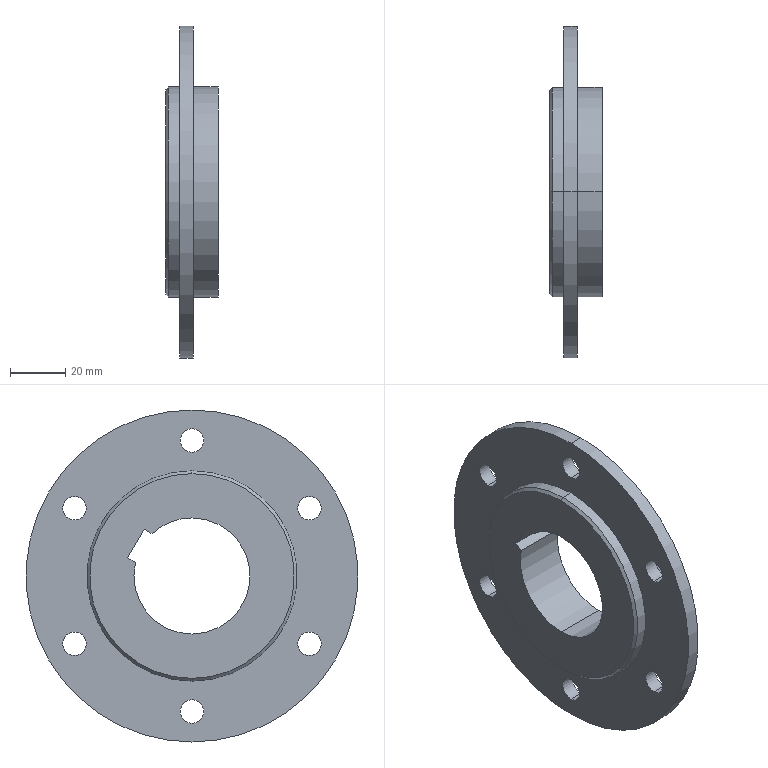Part | SolidWorks | features Chamfer 1, Extrusion 1, HoleWzd 1, ICE 1 | 1 solid | 30 faces | box 19 x 120 x 120 mm | volume 91296 mm3 | cylinder 21 | plane 7 | cone 2 | commonest cylinder face diameters 8.5 x12 76 x4 42 x3 120 x2
STEP:
#1=CARTESIAN_POINT('',(5.,42.435,28.75));
#2=VERTEX_POINT('',#1);
#3=CARTESIAN_POINT('',(5.,42.435,20.25));
#4=VERTEX_POINT('',#3);
#5=CARTESIAN_POINT('',(5.,42.435,24.5));
#6=DIRECTION('',(1.,0.,0.));
#7=DIRECTION('',(0.,0.,-1.));
#8=AXIS2_PLACEMENT_3D('',#5,#6,#7);
#9=CIRCLE('',#8,4.25);
#10=EDGE_CURVE('',#2,#4,#9,.T.);
#11=ORIENTED_EDGE('',*,*,#10,.T.);
#12=CARTESIAN_POINT('',(0.,42.435,20.25));
#13=VERTEX_POINT('',#12);
#14=CARTESIAN_POINT('',(0.,42.435,20.25));
#15=DIRECTION('',(-1.,0.,0.));
#16=VECTOR('',#15,1000.);
#17=LINE('',#14,#16);
#18=EDGE_CURVE('',#4,#13,#17,.T.);
#19=ORIENTED_EDGE('',*,*,#18,.T.);
#20=CARTESIAN_POINT('',(0.,42.435,28.75));
#21=VERTEX_POINT('',#20);
#22=CARTESIAN_POINT('',(0.,42.435,24.5));
#23=DIRECTION('',(-1.,0.,0.));
#24=DIRECTION('',(0.,0.,1.));
#25=AXIS2_PLACEMENT_3D('',#22,#23,#24);
#26=CIRCLE('',#25,4.25);
#27=EDGE_CURVE('',#13,#21,#26,.T.);
#28=ORIENTED_EDGE('',*,*,#27,.T.);
#29=CARTESIAN_POINT('',(0.,42.435,28.75));
#30=DIRECTION('',(-1.,0.,0.));
#31=VECTOR('',#30,1000.);
#32=LINE('',#29,#31);
#33=EDGE_CURVE('',#2,#21,#32,.T.);
#34=ORIENTED_EDGE('',*,*,#33,.F.);
#35=EDGE_LOOP('',(#11,#19,#28,#34));
#36=FACE_OUTER_BOUND('',#35,.T.);
#37=CARTESIAN_POINT('',(0.,42.435,24.5));
#38=DIRECTION('',(-1.,0.,0.));
#39=DIRECTION('',(0.,0.,1.));
#40=AXIS2_PLACEMENT_3D('',#37,#38,#39);
#41=CYLINDRICAL_SURFACE('',#40,4.25);
#42=ADVANCED_FACE('',(#36),#41,.F.);
#43=CARTESIAN_POINT('',(5.,0.,53.25));
#44=VERTEX_POINT('',#43);
#45=CARTESIAN_POINT('',(5.,0.,44.75));
#46=VERTEX_POINT('',#45);
#47=CARTESIAN_POINT('',(5.,0.,49.));
#48=DIRECTION('',(1.,0.,0.));
#49=DIRECTION('',(0.,0.,-1.));
#50=AXIS2_PLACEMENT_3D('',#47,#48,#49);
#51=CIRCLE('',#50,4.25);
#52=EDGE_CURVE('',#44,#46,#51,.T.);
#53=ORIENTED_EDGE('',*,*,#52,.T.);
#54=CARTESIAN_POINT('',(0.,0.,44.75));
#55=VERTEX_POINT('',#54);
#56=CARTESIAN_POINT('',(0.,0.,44.75));
#57=DIRECTION('',(-1.,0.,0.));
#58=VECTOR('',#57,1000.);
#59=LINE('',#56,#58);
#60=EDGE_CURVE('',#46,#55,#59,.T.);
#61=ORIENTED_EDGE('',*,*,#60,.T.);
#62=CARTESIAN_POINT('',(0.,0.,53.25));
#63=VERTEX_POINT('',#62);
#64=CARTESIAN_POINT('',(0.,0.,49.));
#65=DIRECTION('',(-1.,0.,0.));
#66=DIRECTION('',(0.,0.,1.));
#67=AXIS2_PLACEMENT_3D('',#64,#65,#66);
#68=CIRCLE('',#67,4.25);
#69=EDGE_CURVE('',#55,#63,#68,.T.);
#70=ORIENTED_EDGE('',*,*,#69,.T.);
#71=CARTESIAN_POINT('',(0.,0.,53.25));
#72=DIRECTION('',(-1.,0.,0.));
#73=VECTOR('',#72,1000.);
#74=LINE('',#71,#73);
#75=EDGE_CURVE('',#44,#63,#74,.T.);
#76=ORIENTED_EDGE('',*,*,#75,.F.);
#77=EDGE_LOOP('',(#53,#61,#70,#76));
#78=FACE_OUTER_BOUND('',#77,.T.);
#79=CARTESIAN_POINT('',(0.,0.,49.));
#80=DIRECTION('',(-1.,0.,0.));
#81=DIRECTION('',(0.,0.,1.));
#82=AXIS2_PLACEMENT_3D('',#79,#80,#81);
#83=CYLINDRICAL_SURFACE('',#82,4.25);
#84=ADVANCED_FACE('',(#78),#83,.F.);
#85=CARTESIAN_POINT('',(5.,-42.435,28.75));
#86=VERTEX_POINT('',#85);
#87=CARTESIAN_POINT('',(5.,-42.435,20.25));
#88=VERTEX_POINT('',#87);
#89=CARTESIAN_POINT('',(5.,-42.435,24.5));
#90=DIRECTION('',(1.,0.,0.));
#91=DIRECTION('',(0.,0.,-1.));
#92=AXIS2_PLACEMENT_3D('',#89,#90,#91);
#93=CIRCLE('',#92,4.25);
#94=EDGE_CURVE('',#86,#88,#93,.T.);
#95=ORIENTED_EDGE('',*,*,#94,.T.);
#96=CARTESIAN_POINT('',(0.,-42.435,20.25));
#97=VERTEX_POINT('',#96);
#98=CARTESIAN_POINT('',(0.,-42.435,20.25));
#99=DIRECTION('',(-1.,0.,0.));
#100=VECTOR('',#99,1000.);
#101=LINE('',#98,#100);
#102=EDGE_CURVE('',#88,#97,#101,.T.);
#103=ORIENTED_EDGE('',*,*,#102,.T.);
#104=CARTESIAN_POINT('',(0.,-42.435,28.75));
#105=VERTEX_POINT('',#104);
#106=CARTESIAN_POINT('',(0.,-42.435,24.5));
#107=DIRECTION('',(-1.,0.,0.));
#108=DIRECTION('',(0.,0.,1.));
#109=AXIS2_PLACEMENT_3D('',#106,#107,#108);
#110=CIRCLE('',#109,4.25);
#111=EDGE_CURVE('',#97,#105,#110,.T.);
#112=ORIENTED_EDGE('',*,*,#111,.T.);
#113=CARTESIAN_POINT('',(0.,-42.435,28.75));
#114=DIRECTION('',(-1.,0.,0.));
#115=VECTOR('',#114,1000.);
#116=LINE('',#113,#115);
#117=EDGE_CURVE('',#86,#105,#116,.T.);
#118=ORIENTED_EDGE('',*,*,#117,.F.);
#119=EDGE_LOOP('',(#95,#103,#112,#118));
#120=FACE_OUTER_BOUND('',#119,.T.);
#121=CARTESIAN_POINT('',(0.,-42.435,24.5));
#122=DIRECTION('',(-1.,0.,0.));
#123=DIRECTION('',(0.,0.,1.));
#124=AXIS2_PLACEMENT_3D('',#121,#122,#123);
#125=CYLINDRICAL_SURFACE('',#124,4.25);
#126=ADVANCED_FACE('',(#120),#125,.F.);
#127=CARTESIAN_POINT('',(5.,-42.435,-20.25));
#128=VERTEX_POINT('',#127);
#129=CARTESIAN_POINT('',(5.,-42.435,-28.75));
#130=VERTEX_POINT('',#129);
#131=CARTESIAN_POINT('',(5.,-42.435,-24.5));
#132=DIRECTION('',(1.,0.,0.));
#133=DIRECTION('',(0.,0.,-1.));
#134=AXIS2_PLACEMENT_3D('',#131,#132,#133);
#135=CIRCLE('',#134,4.25);
#136=EDGE_CURVE('',#128,#130,#135,.T.);
#137=ORIENTED_EDGE('',*,*,#136,.T.);
#138=CARTESIAN_POINT('',(0.,-42.435,-28.75));
#139=VERTEX_POINT('',#138);
#140=CARTESIAN_POINT('',(0.,-42.435,-28.75));
#141=DIRECTION('',(-1.,0.,0.));
#142=VECTOR('',#141,1000.);
#143=LINE('',#140,#142);
#144=EDGE_CURVE('',#130,#139,#143,.T.);
#145=ORIENTED_EDGE('',*,*,#144,.T.);
#146=CARTESIAN_POINT('',(0.,-42.435,-20.25));
#147=VERTEX_POINT('',#146);
#148=CARTESIAN_POINT('',(0.,-42.435,-24.5));
#149=DIRECTION('',(-1.,0.,0.));
#150=DIRECTION('',(0.,0.,1.));
#151=AXIS2_PLACEMENT_3D('',#148,#149,#150);
#152=CIRCLE('',#151,4.25);
#153=EDGE_CURVE('',#139,#147,#152,.T.);
#154=ORIENTED_EDGE('',*,*,#153,.T.);
#155=CARTESIAN_POINT('',(0.,-42.435,-20.25));
#156=DIRECTION('',(-1.,0.,0.));
#157=VECTOR('',#156,1000.);
#158=LINE('',#155,#157);
#159=EDGE_CURVE('',#128,#147,#158,.T.);
#160=ORIENTED_EDGE('',*,*,#159,.F.);
#161=EDGE_LOOP('',(#137,#145,#154,#160));
#162=FACE_OUTER_BOUND('',#161,.T.);
#163=CARTESIAN_POINT('',(0.,-42.435,-24.5));
#164=DIRECTION('',(-1.,0.,0.));
#165=DIRECTION('',(0.,0.,1.));
#166=AXIS2_PLACEMENT_3D('',#163,#164,#165);
#167=CYLINDRICAL_SURFACE('',#166,4.25);
#168=ADVANCED_FACE('',(#162),#167,.F.);
#169=CARTESIAN_POINT('',(5.,0.,-44.75));
#170=VERTEX_POINT('',#169);
#171=CARTESIAN_POINT('',(5.,0.,-53.25));
#172=VERTEX_POINT('',#171);
#173=CARTESIAN_POINT('',(5.,0.,-49.));
#174=DIRECTION('',(1.,0.,0.));
#175=DIRECTION('',(0.,0.,-1.));
#176=AXIS2_PLACEMENT_3D('',#173,#174,#175);
#177=CIRCLE('',#176,4.25);
#178=EDGE_CURVE('',#170,#172,#177,.T.);
#179=ORIENTED_EDGE('',*,*,#178,.T.);
#180=CARTESIAN_POINT('',(0.,0.,-53.25));
#181=VERTEX_POINT('',#180);
#182=CARTESIAN_POINT('',(0.,0.,-53.25));
#183=DIRECTION('',(-1.,0.,0.));
#184=VECTOR('',#183,1000.);
#185=LINE('',#182,#184);
#186=EDGE_CURVE('',#172,#181,#185,.T.);
#187=ORIENTED_EDGE('',*,*,#186,.T.);
#188=CARTESIAN_POINT('',(0.,0.,-44.75));
#189=VERTEX_POINT('',#188);
#190=CARTESIAN_POINT('',(0.,0.,-49.));
#191=DIRECTION('',(-1.,0.,0.));
#192=DIRECTION('',(0.,0.,1.));
#193=AXIS2_PLACEMENT_3D('',#190,#191,#192);
#194=CIRCLE('',#193,4.25);
#195=EDGE_CURVE('',#181,#189,#194,.T.);
#196=ORIENTED_EDGE('',*,*,#195,.T.);
#197=CARTESIAN_POINT('',(0.,0.,-44.75));
#198=DIRECTION('',(-1.,0.,0.));
#199=VECTOR('',#198,1000.);
#200=LINE('',#197,#199);
#201=EDGE_CURVE('',#170,#189,#200,.T.);
#202=ORIENTED_EDGE('',*,*,#201,.F.);
#203=EDGE_LOOP('',(#179,#187,#196,#202));
#204=FACE_OUTER_BOUND('',#203,.T.);
#205=CARTESIAN_POINT('',(0.,0.,-49.));
#206=DIRECTION('',(-1.,0.,0.));
#207=DIRECTION('',(0.,0.,1.));
#208=AXIS2_PLACEMENT_3D('',#205,#206,#207);
#209=CYLINDRICAL_SURFACE('',#208,4.25);
#210=ADVANCED_FACE('',(#204),#209,.F.);
#211=CARTESIAN_POINT('',(5.,42.435,-20.25));
#212=VERTEX_POINT('',#211);
#213=CARTESIAN_POINT('',(5.,42.435,-28.75));
#214=VERTEX_POINT('',#213);
#215=CARTESIAN_POINT('',(5.,42.435,-24.5));
#216=DIRECTION('',(1.,0.,0.));
#217=DIRECTION('',(0.,0.,-1.));
#218=AXIS2_PLACEMENT_3D('',#215,#216,#217);
#219=CIRCLE('',#218,4.25);
#220=EDGE_CURVE('',#212,#214,#219,.T.);
#221=ORIENTED_EDGE('',*,*,#220,.T.);
#222=CARTESIAN_POINT('',(0.,42.435,-28.75));
#223=VERTEX_POINT('',#222);
#224=CARTESIAN_POINT('',(0.,42.435,-28.75));
#225=DIRECTION('',(-1.,0.,0.));
#226=VECTOR('',#225,1000.);
#227=LINE('',#224,#226);
#228=EDGE_CURVE('',#214,#223,#227,.T.);
#229=ORIENTED_EDGE('',*,*,#228,.T.);
#230=CARTESIAN_POINT('',(0.,42.435,-20.25));
#231=VERTEX_POINT('',#230);
#232=CARTESIAN_POINT('',(0.,42.435,-24.5));
#233=DIRECTION('',(-1.,0.,0.));
#234=DIRECTION('',(0.,0.,1.));
#235=AXIS2_PLACEMENT_3D('',#232,#233,#234);
#236=CIRCLE('',#235,4.25);
#237=EDGE_CURVE('',#223,#231,#236,.T.);
#238=ORIENTED_EDGE('',*,*,#237,.T.);
#239=CARTESIAN_POINT('',(0.,42.435,-20.25));
#240=DIRECTION('',(-1.,0.,0.));
#241=VECTOR('',#240,1000.);
#242=LINE('',#239,#241);
#243=EDGE_CURVE('',#212,#231,#242,.T.);
#244=ORIENTED_EDGE('',*,*,#243,.F.);
#245=EDGE_LOOP('',(#221,#229,#238,#244));
#246=FACE_OUTER_BOUND('',#245,.T.);
#247=CARTESIAN_POINT('',(0.,42.435,-24.5));
#248=DIRECTION('',(-1.,0.,0.));
#249=DIRECTION('',(0.,0.,1.));
#250=AXIS2_PLACEMENT_3D('',#247,#248,#249);
#251=CYLINDRICAL_SURFACE('',#250,4.25);
#252=ADVANCED_FACE('',(#246),#251,.F.);
#253=CARTESIAN_POINT('',(-5.,0.,37.));
#254=VERTEX_POINT('',#253);
#255=CARTESIAN_POINT('',(-5.,0.,-37.));
#256=VERTEX_POINT('',#255);
#257=CARTESIAN_POINT('',(-5.,0.,0.));
#258=DIRECTION('',(-1.,0.,0.));
#259=DIRECTION('',(0.,0.,-1.));
#260=AXIS2_PLACEMENT_3D('',#257,#258,#259);
#261=CIRCLE('',#260,37.);
#262=EDGE_CURVE('',#254,#256,#261,.T.);
#263=ORIENTED_EDGE('',*,*,#262,.F.);
#264=CARTESIAN_POINT('',(-4.,0.,38.));
#265=VERTEX_POINT('',#264);
#266=CARTESIAN_POINT('',(-4.,0.,38.));
#267=DIRECTION('',(0.7071,0.,0.7071));
#268=VECTOR('',#267,1000.);
#269=LINE('',#266,#268);
#270=EDGE_CURVE('',#254,#265,#269,.T.);
#271=ORIENTED_EDGE('',*,*,#270,.T.);
#272=CARTESIAN_POINT('',(-4.,0.,-38.));
#273=VERTEX_POINT('',#272);
#274=CARTESIAN_POINT('',(-4.,0.,0.));
#275=DIRECTION('',(1.,0.,0.));
#276=DIRECTION('',(0.,0.,-1.));
#277=AXIS2_PLACEMENT_3D('',#274,#275,#276);
#278=CIRCLE('',#277,38.);
#279=EDGE_CURVE('',#273,#265,#278,.T.);
#280=ORIENTED_EDGE('',*,*,#279,.F.);
#281=CARTESIAN_POINT('',(-4.,0.,-38.));
#282=DIRECTION('',(0.7071,0.,-0.7071));
#283=VECTOR('',#282,1000.);
#284=LINE('',#281,#283);
#285=EDGE_CURVE('',#256,#273,#284,.T.);
#286=ORIENTED_EDGE('',*,*,#285,.F.);
#287=EDGE_LOOP('',(#263,#271,#280,#286));
#288=FACE_OUTER_BOUND('',#287,.T.);
#289=CARTESIAN_POINT('',(-4.,0.,0.));
#290=DIRECTION('',(1.,0.,0.));
#291=DIRECTION('',(0.,0.,-1.));
#292=AXIS2_PLACEMENT_3D('',#289,#290,#291);
#293=CONICAL_SURFACE('',#292,38.,0.7854);
#294=ADVANCED_FACE('',(#288),#293,.T.);
#295=CARTESIAN_POINT('',(5.,0.,-60.));
#296=VERTEX_POINT('',#295);
#297=CARTESIAN_POINT('',(5.,0.,60.));
#298=VERTEX_POINT('',#297);
#299=CARTESIAN_POINT('',(5.,0.,0.));
#300=DIRECTION('',(1.,0.,0.));
#301=DIRECTION('',(0.,0.,-1.));
#302=AXIS2_PLACEMENT_3D('',#299,#300,#301);
#303=CIRCLE('',#302,60.);
#304=EDGE_CURVE('',#296,#298,#303,.T.);
#305=ORIENTED_EDGE('',*,*,#304,.F.);
#306=CARTESIAN_POINT('',(0.,0.,-60.));
#307=VERTEX_POINT('',#306);
#308=CARTESIAN_POINT('',(5.,0.,-60.));
#309=DIRECTION('',(-1.,0.,0.));
#310=VECTOR('',#309,1000.);
#311=LINE('',#308,#310);
#312=EDGE_CURVE('',#296,#307,#311,.T.);
#313=ORIENTED_EDGE('',*,*,#312,.T.);
#314=CARTESIAN_POINT('',(0.,0.,60.));
#315=VERTEX_POINT('',#314);
#316=CARTESIAN_POINT('',(0.,0.,0.));
#317=DIRECTION('',(1.,0.,0.));
#318=DIRECTION('',(0.,0.,-1.));
#319=AXIS2_PLACEMENT_3D('',#316,#317,#318);
#320=CIRCLE('',#319,60.);
#321=EDGE_CURVE('',#307,#315,#320,.T.);
#322=ORIENTED_EDGE('',*,*,#321,.T.);
#323=CARTESIAN_POINT('',(5.,0.,60.));
#324=DIRECTION('',(-1.,0.,0.));
#325=VECTOR('',#324,1000.);
#326=LINE('',#323,#325);
#327=EDGE_CURVE('',#298,#315,#326,.T.);
#328=ORIENTED_EDGE('',*,*,#327,.F.);
#329=EDGE_LOOP('',(#305,#313,#322,#328));
#330=FACE_OUTER_BOUND('',#329,.T.);
#331=CARTESIAN_POINT('',(5.,0.,0.));
#332=DIRECTION('',(-1.,0.,0.));
#333=DIRECTION('',(0.,0.,1.));
#334=AXIS2_PLACEMENT_3D('',#331,#332,#333);
#335=CYLINDRICAL_SURFACE('',#334,60.);
#336=ADVANCED_FACE('',(#330),#335,.T.);
#337=CARTESIAN_POINT('',(-5.,0.,21.));
#338=VERTEX_POINT('',#337);
#339=CARTESIAN_POINT('',(-5.,0.,-21.));
#340=VERTEX_POINT('',#339);
#341=CARTESIAN_POINT('',(-5.,0.,0.));
#342=DIRECTION('',(1.,0.,0.));
#343=DIRECTION('',(0.,0.,-1.));
#344=AXIS2_PLACEMENT_3D('',#341,#342,#343);
#345=CIRCLE('',#344,21.);
#346=EDGE_CURVE('',#338,#340,#345,.T.);
#347=ORIENTED_EDGE('',*,*,#346,.F.);
#348=CARTESIAN_POINT('',(14.,0.,21.));
#349=VERTEX_POINT('',#348);
#350=CARTESIAN_POINT('',(-5.,0.,21.));
#351=DIRECTION('',(1.,0.,0.));
#352=VECTOR('',#351,1000.);
#353=LINE('',#350,#352);
#354=EDGE_CURVE('',#338,#349,#353,.T.);
#355=ORIENTED_EDGE('',*,*,#354,.T.);
#356=CARTESIAN_POINT('',(14.,0.,-21.));
#357=VERTEX_POINT('',#356);
#358=CARTESIAN_POINT('',(14.,0.,0.));
#359=DIRECTION('',(1.,0.,0.));
#360=DIRECTION('',(0.,0.,-1.));
#361=AXIS2_PLACEMENT_3D('',#358,#359,#360);
#362=CIRCLE('',#361,21.);
#363=EDGE_CURVE('',#349,#357,#362,.T.);
#364=ORIENTED_EDGE('',*,*,#363,.T.);
#365=CARTESIAN_POINT('',(-5.,0.,-21.));
#366=DIRECTION('',(1.,0.,0.));
#367=VECTOR('',#366,1000.);
#368=LINE('',#365,#367);
#369=EDGE_CURVE('',#340,#357,#368,.T.);
#370=ORIENTED_EDGE('',*,*,#369,.F.);
#371=EDGE_LOOP('',(#347,#355,#364,#370));
#372=FACE_OUTER_BOUND('',#371,.T.);
#373=CARTESIAN_POINT('',(-5.,0.,0.));
#374=DIRECTION('',(1.,0.,0.));
#375=DIRECTION('',(0.,0.,-1.));
#376=AXIS2_PLACEMENT_3D('',#373,#374,#375);
#377=CYLINDRICAL_SURFACE('',#376,21.);
#378=ADVANCED_FACE('',(#372),#377,.F.);
#379=CARTESIAN_POINT('',(-5.,20.428,4.866));
#380=VERTEX_POINT('',#379);
#381=CARTESIAN_POINT('',(-5.,0.,0.));
#382=DIRECTION('',(1.,0.,0.));
#383=DIRECTION('',(0.,0.,-1.));
#384=AXIS2_PLACEMENT_3D('',#381,#382,#383);
#385=CIRCLE('',#384,21.);
#386=EDGE_CURVE('',#340,#380,#385,.T.);
#387=ORIENTED_EDGE('',*,*,#386,.F.);
#388=ORIENTED_EDGE('',*,*,#369,.T.);
#389=CARTESIAN_POINT('',(14.,20.428,4.866));
#390=VERTEX_POINT('',#389);
#391=CARTESIAN_POINT('',(14.,0.,0.));
#392=DIRECTION('',(1.,0.,0.));
#393=DIRECTION('',(0.,0.,-1.));
#394=AXIS2_PLACEMENT_3D('',#391,#392,#393);
#395=CIRCLE('',#394,21.);
#396=EDGE_CURVE('',#357,#390,#395,.T.);
#397=ORIENTED_EDGE('',*,*,#396,.T.);
#398=CARTESIAN_POINT('',(-5.,20.428,4.866));
#399=DIRECTION('',(1.,0.,0.));
#400=VECTOR('',#399,1000.);
#401=LINE('',#398,#400);
#402=EDGE_CURVE('',#380,#390,#401,.T.);
#403=ORIENTED_EDGE('',*,*,#402,.F.);
#404=EDGE_LOOP('',(#387,#388,#397,#403));
#405=FACE_OUTER_BOUND('',#404,.T.);
#406=CARTESIAN_POINT('',(-5.,0.,0.));
#407=DIRECTION('',(1.,0.,0.));
#408=DIRECTION('',(0.,0.,-1.));
#409=AXIS2_PLACEMENT_3D('',#406,#407,#408);
#410=CYLINDRICAL_SURFACE('',#409,21.);
#411=ADVANCED_FACE('',(#405),#410,.F.);
#412=CARTESIAN_POINT('',(5.,0.,38.));
#413=VERTEX_POINT('',#412);
#414=CARTESIAN_POINT('',(5.,0.,-38.));
#415=VERTEX_POINT('',#414);
#416=CARTESIAN_POINT('',(5.,0.,0.));
#417=DIRECTION('',(-1.,0.,0.));
#418=DIRECTION('',(0.,0.,-1.));
#419=AXIS2_PLACEMENT_3D('',#416,#417,#418);
#420=CIRCLE('',#419,38.);
#421=EDGE_CURVE('',#413,#415,#420,.T.);
#422=ORIENTED_EDGE('',*,*,#421,.F.);
#423=CARTESIAN_POINT('',(14.,0.,38.));
#424=VERTEX_POINT('',#423);
#425=CARTESIAN_POINT('',(-5.,0.,38.));
#426=DIRECTION('',(1.,0.,0.));
#427=VECTOR('',#426,1000.);
#428=LINE('',#425,#427);
#429=EDGE_CURVE('',#413,#424,#428,.T.);
#430=ORIENTED_EDGE('',*,*,#429,.T.);
#431=CARTESIAN_POINT('',(14.,0.,-38.));
#432=VERTEX_POINT('',#431);
#433=CARTESIAN_POINT('',(14.,0.,0.));
#434=DIRECTION('',(1.,0.,0.));
#435=DIRECTION('',(0.,0.,-1.));
#436=AXIS2_PLACEMENT_3D('',#433,#434,#435);
#437=CIRCLE('',#436,38.);
#438=EDGE_CURVE('',#432,#424,#437,.T.);
#439=ORIENTED_EDGE('',*,*,#438,.F.);
#440=CARTESIAN_POINT('',(-5.,0.,-38.));
#441=DIRECTION('',(1.,0.,0.));
#442=VECTOR('',#441,1000.);
#443=LINE('',#440,#442);
#444=EDGE_CURVE('',#415,#432,#443,.T.);
#445=ORIENTED_EDGE('',*,*,#444,.F.);
#446=EDGE_LOOP('',(#422,#430,#439,#445));
#447=FACE_OUTER_BOUND('',#446,.T.);
#448=CARTESIAN_POINT('',(-5.,0.,0.));
#449=DIRECTION('',(1.,0.,0.));
#450=DIRECTION('',(0.,0.,-1.));
#451=AXIS2_PLACEMENT_3D('',#448,#449,#450);
#452=CYLINDRICAL_SURFACE('',#451,38.);
#453=ADVANCED_FACE('',(#447),#452,.T.);
#454=ORIENTED_EDGE('',*,*,#279,.T.);
#455=CARTESIAN_POINT('',(0.,0.,38.));
#456=VERTEX_POINT('',#455);
#457=CARTESIAN_POINT('',(-5.,0.,38.));
#458=DIRECTION('',(1.,0.,0.));
#459=VECTOR('',#458,1000.);
#460=LINE('',#457,#459);
#461=EDGE_CURVE('',#265,#456,#460,.T.);
#462=ORIENTED_EDGE('',*,*,#461,.T.);
#463=CARTESIAN_POINT('',(0.,0.,-38.));
#464=VERTEX_POINT('',#463);
#465=CARTESIAN_POINT('',(0.,0.,0.));
#466=DIRECTION('',(1.,0.,0.));
#467=DIRECTION('',(0.,0.,-1.));
#468=AXIS2_PLACEMENT_3D('',#465,#466,#467);
#469=CIRCLE('',#468,38.);
#470=EDGE_CURVE('',#464,#456,#469,.T.);
#471=ORIENTED_EDGE('',*,*,#470,.F.);
#472=CARTESIAN_POINT('',(-5.,0.,-38.));
#473=DIRECTION('',(1.,0.,0.));
#474=VECTOR('',#473,1000.);
#475=LINE('',#472,#474);
#476=EDGE_CURVE('',#273,#464,#475,.T.);
#477=ORIENTED_EDGE('',*,*,#476,.F.);
#478=EDGE_LOOP('',(#454,#462,#471,#477));
#479=FACE_OUTER_BOUND('',#478,.T.);
#480=CARTESIAN_POINT('',(-5.,0.,0.));
#481=DIRECTION('',(1.,0.,0.));
#482=DIRECTION('',(0.,0.,-1.));
#483=AXIS2_PLACEMENT_3D('',#480,#481,#482);
#484=CYLINDRICAL_SURFACE('',#483,38.);
#485=ADVANCED_FACE('',(#479),#484,.T.);
#486=ORIENTED_EDGE('',*,*,#461,.F.);
#487=CARTESIAN_POINT('',(-4.,0.,0.));
#488=DIRECTION('',(1.,0.,0.));
#489=DIRECTION('',(0.,0.,-1.));
#490=AXIS2_PLACEMENT_3D('',#487,#488,#489);
#491=CIRCLE('',#490,38.);
#492=EDGE_CURVE('',#265,#273,#491,.T.);
#493=ORIENTED_EDGE('',*,*,#492,.T.);
#494=ORIENTED_EDGE('',*,*,#476,.T.);
#495=CARTESIAN_POINT('',(0.,0.,0.));
#496=DIRECTION('',(1.,0.,0.));
#497=DIRECTION('',(0.,0.,-1.));
#498=AXIS2_PLACEMENT_3D('',#495,#496,#497);
#499=CIRCLE('',#498,38.);
#500=EDGE_CURVE('',#456,#464,#499,.T.);
#501=ORIENTED_EDGE('',*,*,#500,.F.);
#502=EDGE_LOOP('',(#486,#493,#494,#501));
#503=FACE_OUTER_BOUND('',#502,.T.);
#504=CARTESIAN_POINT('',(-5.,0.,0.));
#505=DIRECTION('',(1.,0.,0.));
#506=DIRECTION('',(0.,0.,-1.));
#507=AXIS2_PLACEMENT_3D('',#504,#505,#506);
#508=CYLINDRICAL_SURFACE('',#507,38.);
#509=ADVANCED_FACE('',(#503),#508,.T.);
#510=ORIENTED_EDGE('',*,*,#429,.F.);
#511=CARTESIAN_POINT('',(5.,0.,0.));
#512=DIRECTION('',(-1.,0.,0.));
#513=DIRECTION('',(0.,0.,-1.));
#514=AXIS2_PLACEMENT_3D('',#511,#512,#513);
#515=CIRCLE('',#514,38.);
#516=EDGE_CURVE('',#415,#413,#515,.T.);
#517=ORIENTED_EDGE('',*,*,#516,.F.);
#518=ORIENTED_EDGE('',*,*,#444,.T.);
#519=CARTESIAN_POINT('',(14.,0.,0.));
#520=DIRECTION('',(1.,0.,0.));
#521=DIRECTION('',(0.,0.,-1.));
#522=AXIS2_PLACEMENT_3D('',#519,#520,#521);
#523=CIRCLE('',#522,38.);
#524=EDGE_CURVE('',#424,#432,#523,.T.);
#525=ORIENTED_EDGE('',*,*,#524,.F.);
#526=EDGE_LOOP('',(#510,#517,#518,#525));
#527=FACE_OUTER_BOUND('',#526,.T.);
#528=CARTESIAN_POINT('',(-5.,0.,0.));
#529=DIRECTION('',(1.,0.,0.));
#530=DIRECTION('',(0.,0.,-1.));
#531=AXIS2_PLACEMENT_3D('',#528,#529,#530);
#532=CYLINDRICAL_SURFACE('',#531,38.);
#533=ADVANCED_FACE('',(#527),#532,.T.);
#534=CARTESIAN_POINT('',(-5.,0.,0.));
#535=DIRECTION('',(-1.,0.,0.));
#536=DIRECTION('',(0.,0.,-1.));
#537=AXIS2_PLACEMENT_3D('',#534,#535,#536);
#538=CIRCLE('',#537,37.);
#539=EDGE_CURVE('',#256,#254,#538,.T.);
#540=ORIENTED_EDGE('',*,*,#539,.T.);
#541=ORIENTED_EDGE('',*,*,#262,.T.);
#542=EDGE_LOOP('',(#540,#541));
#543=FACE_OUTER_BOUND('',#542,.T.);
#544=CARTESIAN_POINT('',(-5.,17.286,16.908));
#545=VERTEX_POINT('',#544);
#546=CARTESIAN_POINT('',(-5.,14.428,15.258));
#547=VERTEX_POINT('',#546);
#548=CARTESIAN_POINT('',(-5.,17.286,16.908));
#549=DIRECTION('',(0.,-0.866,-0.5));
#550=VECTOR('',#549,1000.);
#551=LINE('',#548,#550);
#552=EDGE_CURVE('',#545,#547,#551,.T.);
#553=ORIENTED_EDGE('',*,*,#552,.T.);
#554=CARTESIAN_POINT('',(-5.,0.,0.));
#555=DIRECTION('',(1.,0.,0.));
#556=DIRECTION('',(0.,0.,-1.));
#557=AXIS2_PLACEMENT_3D('',#554,#555,#556);
#558=CIRCLE('',#557,21.);
#559=EDGE_CURVE('',#547,#338,#558,.T.);
#560=ORIENTED_EDGE('',*,*,#559,.T.);
#561=ORIENTED_EDGE('',*,*,#346,.T.);
#562=ORIENTED_EDGE('',*,*,#386,.T.);
#563=CARTESIAN_POINT('',(-5.,23.286,6.516));
#564=VERTEX_POINT('',#563);
#565=CARTESIAN_POINT('',(-5.,20.428,4.866));
#566=DIRECTION('',(0.,0.866,0.5));
#567=VECTOR('',#566,1000.);
#568=LINE('',#565,#567);
#569=EDGE_CURVE('',#380,#564,#568,.T.);
#570=ORIENTED_EDGE('',*,*,#569,.T.);
#571=CARTESIAN_POINT('',(-5.,23.286,6.516));
#572=DIRECTION('',(0.,-0.5,0.866));
#573=VECTOR('',#572,1000.);
#574=LINE('',#571,#573);
#575=EDGE_CURVE('',#564,#545,#574,.T.);
#576=ORIENTED_EDGE('',*,*,#575,.T.);
#577=EDGE_LOOP('',(#553,#560,#561,#562,#570,#576));
#578=FACE_BOUND('',#577,.T.);
#579=CARTESIAN_POINT('',(-5.,0.,0.));
#580=DIRECTION('',(1.,0.,0.));
#581=DIRECTION('',(0.,0.,-1.));
#582=AXIS2_PLACEMENT_3D('',#579,#580,#581);
#583=PLANE('',#582);
#584=ADVANCED_FACE('',(#543,#578),#583,.F.);
#585=ORIENTED_EDGE('',*,*,#354,.F.);
#586=ORIENTED_EDGE('',*,*,#559,.F.);
#587=CARTESIAN_POINT('',(14.,14.428,15.258));
#588=VERTEX_POINT('',#587);
#589=CARTESIAN_POINT('',(-5.,14.428,15.258));
#590=DIRECTION('',(1.,0.,0.));
#591=VECTOR('',#590,1000.);
#592=LINE('',#589,#591);
#593=EDGE_CURVE('',#547,#588,#592,.T.);
#594=ORIENTED_EDGE('',*,*,#593,.T.);
#595=CARTESIAN_POINT('',(14.,0.,0.));
#596=DIRECTION('',(1.,0.,0.));
#597=DIRECTION('',(0.,0.,-1.));
#598=AXIS2_PLACEMENT_3D('',#595,#596,#597);
#599=CIRCLE('',#598,21.);
#600=EDGE_CURVE('',#588,#349,#599,.T.);
#601=ORIENTED_EDGE('',*,*,#600,.T.);
#602=EDGE_LOOP('',(#585,#586,#594,#601));
#603=FACE_OUTER_BOUND('',#602,.T.);
#604=CARTESIAN_POINT('',(-5.,0.,0.));
#605=DIRECTION('',(1.,0.,0.));
#606=DIRECTION('',(0.,0.,-1.));
#607=AXIS2_PLACEMENT_3D('',#604,#605,#606);
#608=CYLINDRICAL_SURFACE('',#607,21.);
#609=ADVANCED_FACE('',(#603),#608,.F.);
#610=CARTESIAN_POINT('',(14.,17.286,16.908));
#611=VERTEX_POINT('',#610);
#612=CARTESIAN_POINT('',(-5.,17.286,16.908));
#613=DIRECTION('',(1.,0.,0.));
#614=VECTOR('',#613,1000.);
#615=LINE('',#612,#614);
#616=EDGE_CURVE('',#545,#611,#615,.T.);
#617=ORIENTED_EDGE('',*,*,#616,.T.);
#618=CARTESIAN_POINT('',(14.,17.286,16.908));
#619=DIRECTION('',(0.,-0.866,-0.5));
#620=VECTOR('',#619,1000.);
#621=LINE('',#618,#620);
#622=EDGE_CURVE('',#611,#588,#621,.T.);
#623=ORIENTED_EDGE('',*,*,#622,.T.);
#624=ORIENTED_EDGE('',*,*,#593,.F.);
#625=ORIENTED_EDGE('',*,*,#552,.F.);
#626=EDGE_LOOP('',(#617,#623,#624,#625));
#627=FACE_OUTER_BOUND('',#626,.T.);
#628=CARTESIAN_POINT('',(-5.,17.286,16.908));
#629=DIRECTION('',(0.,-0.5,0.866));
#630=DIRECTION('',(0.,-0.866,-0.5));
#631=AXIS2_PLACEMENT_3D('',#628,#629,#630);
#632=PLANE('',#631);
#633=ADVANCED_FACE('',(#627),#632,.F.);
#634=CARTESIAN_POINT('',(14.,23.286,6.516));
#635=VERTEX_POINT('',#634);
#636=CARTESIAN_POINT('',(-5.,23.286,6.516));
#637=DIRECTION('',(1.,0.,0.));
#638=VECTOR('',#637,1000.);
#639=LINE('',#636,#638);
#640=EDGE_CURVE('',#564,#635,#639,.T.);
#641=ORIENTED_EDGE('',*,*,#640,.T.);
#642=CARTESIAN_POINT('',(14.,23.286,6.516));
#643=DIRECTION('',(0.,-0.5,0.866));
#644=VECTOR('',#643,1000.);
#645=LINE('',#642,#644);
#646=EDGE_CURVE('',#635,#611,#645,.T.);
#647=ORIENTED_EDGE('',*,*,#646,.T.);
#648=ORIENTED_EDGE('',*,*,#616,.F.);
#649=ORIENTED_EDGE('',*,*,#575,.F.);
#650=EDGE_LOOP('',(#641,#647,#648,#649));
#651=FACE_OUTER_BOUND('',#650,.T.);
#652=CARTESIAN_POINT('',(-5.,23.286,6.516));
#653=DIRECTION('',(0.,0.866,0.5));
#654=DIRECTION('',(0.,-0.5,0.866));
#655=AXIS2_PLACEMENT_3D('',#652,#653,#654);
#656=PLANE('',#655);
#657=ADVANCED_FACE('',(#651),#656,.F.);
#658=ORIENTED_EDGE('',*,*,#402,.T.);
#659=CARTESIAN_POINT('',(14.,20.428,4.866));
#660=DIRECTION('',(0.,0.866,0.5));
#661=VECTOR('',#660,1000.);
#662=LINE('',#659,#661);
#663=EDGE_CURVE('',#390,#635,#662,.T.);
#664=ORIENTED_EDGE('',*,*,#663,.T.);
#665=ORIENTED_EDGE('',*,*,#640,.F.);
#666=ORIENTED_EDGE('',*,*,#569,.F.);
#667=EDGE_LOOP('',(#658,#664,#665,#666));
#668=FACE_OUTER_BOUND('',#667,.T.);
#669=CARTESIAN_POINT('',(-5.,20.428,4.866));
#670=DIRECTION('',(0.,0.5,-0.866));
#671=DIRECTION('',(0.,0.866,0.5));
#672=AXIS2_PLACEMENT_3D('',#669,#670,#671);
#673=PLANE('',#672);
#674=ADVANCED_FACE('',(#668),#673,.F.);
#675=ORIENTED_EDGE('',*,*,#438,.T.);
#676=ORIENTED_EDGE('',*,*,#524,.T.);
#677=EDGE_LOOP('',(#675,#676));
#678=FACE_OUTER_BOUND('',#677,.T.);
#679=ORIENTED_EDGE('',*,*,#663,.F.);
#680=ORIENTED_EDGE('',*,*,#396,.F.);
#681=ORIENTED_EDGE('',*,*,#363,.F.);
#682=ORIENTED_EDGE('',*,*,#600,.F.);
#683=ORIENTED_EDGE('',*,*,#622,.F.);
#684=ORIENTED_EDGE('',*,*,#646,.F.);
#685=EDGE_LOOP('',(#679,#680,#681,#682,#683,#684));
#686=FACE_BOUND('',#685,.T.);
#687=CARTESIAN_POINT('',(14.,0.,0.));
#688=DIRECTION('',(1.,0.,0.));
#689=DIRECTION('',(0.,0.,-1.));
#690=AXIS2_PLACEMENT_3D('',#687,#688,#689);
#691=PLANE('',#690);
#692=ADVANCED_FACE('',(#678,#686),#691,.T.);
#693=ORIENTED_EDGE('',*,*,#10,.F.);
#694=CARTESIAN_POINT('',(5.,42.435,24.5));
#695=DIRECTION('',(1.,0.,0.));
#696=DIRECTION('',(0.,0.,-1.));
#697=AXIS2_PLACEMENT_3D('',#694,#695,#696);
#698=CIRCLE('',#697,4.25);
#699=EDGE_CURVE('',#4,#2,#698,.T.);
#700=ORIENTED_EDGE('',*,*,#699,.F.);
#701=EDGE_LOOP('',(#693,#700));
#702=FACE_BOUND('',#701,.T.);
#703=ORIENTED_EDGE('',*,*,#52,.F.);
#704=CARTESIAN_POINT('',(5.,0.,49.));
#705=DIRECTION('',(1.,0.,0.));
#706=DIRECTION('',(0.,0.,-1.));
#707=AXIS2_PLACEMENT_3D('',#704,#705,#706);
#708=CIRCLE('',#707,4.25);
#709=EDGE_CURVE('',#46,#44,#708,.T.);
#710=ORIENTED_EDGE('',*,*,#709,.F.);
#711=EDGE_LOOP('',(#703,#710));
#712=FACE_BOUND('',#711,.T.);
#713=ORIENTED_EDGE('',*,*,#94,.F.);
#714=CARTESIAN_POINT('',(5.,-42.435,24.5));
#715=DIRECTION('',(1.,0.,0.));
#716=DIRECTION('',(0.,0.,-1.));
#717=AXIS2_PLACEMENT_3D('',#714,#715,#716);
#718=CIRCLE('',#717,4.25);
#719=EDGE_CURVE('',#88,#86,#718,.T.);
#720=ORIENTED_EDGE('',*,*,#719,.F.);
#721=EDGE_LOOP('',(#713,#720));
#722=FACE_BOUND('',#721,.T.);
#723=ORIENTED_EDGE('',*,*,#136,.F.);
#724=CARTESIAN_POINT('',(5.,-42.435,-24.5));
#725=DIRECTION('',(1.,0.,0.));
#726=DIRECTION('',(0.,0.,-1.));
#727=AXIS2_PLACEMENT_3D('',#724,#725,#726);
#728=CIRCLE('',#727,4.25);
#729=EDGE_CURVE('',#130,#128,#728,.T.);
#730=ORIENTED_EDGE('',*,*,#729,.F.);
#731=EDGE_LOOP('',(#723,#730));
#732=FACE_BOUND('',#731,.T.);
#733=ORIENTED_EDGE('',*,*,#178,.F.);
#734=CARTESIAN_POINT('',(5.,0.,-49.));
#735=DIRECTION('',(1.,0.,0.));
#736=DIRECTION('',(0.,0.,-1.));
#737=AXIS2_PLACEMENT_3D('',#734,#735,#736);
#738=CIRCLE('',#737,4.25);
#739=EDGE_CURVE('',#172,#170,#738,.T.);
#740=ORIENTED_EDGE('',*,*,#739,.F.);
#741=EDGE_LOOP('',(#733,#740));
#742=FACE_BOUND('',#741,.T.);
#743=ORIENTED_EDGE('',*,*,#220,.F.);
#744=CARTESIAN_POINT('',(5.,42.435,-24.5));
#745=DIRECTION('',(1.,0.,0.));
#746=DIRECTION('',(0.,0.,-1.));
#747=AXIS2_PLACEMENT_3D('',#744,#745,#746);
#748=CIRCLE('',#747,4.25);
#749=EDGE_CURVE('',#214,#212,#748,.T.);
#750=ORIENTED_EDGE('',*,*,#749,.F.);
#751=EDGE_LOOP('',(#743,#750));
#752=FACE_BOUND('',#751,.T.);
#753=CARTESIAN_POINT('',(5.,0.,0.));
#754=DIRECTION('',(1.,0.,0.));
#755=DIRECTION('',(0.,0.,-1.));
#756=AXIS2_PLACEMENT_3D('',#753,#754,#755);
#757=CIRCLE('',#756,60.);
#758=EDGE_CURVE('',#298,#296,#757,.T.);
#759=ORIENTED_EDGE('',*,*,#758,.T.);
#760=ORIENTED_EDGE('',*,*,#304,.T.);
#761=EDGE_LOOP('',(#759,#760));
#762=FACE_OUTER_BOUND('',#761,.T.);
#763=ORIENTED_EDGE('',*,*,#516,.T.);
#764=ORIENTED_EDGE('',*,*,#421,.T.);
#765=EDGE_LOOP('',(#763,#764));
#766=FACE_BOUND('',#765,.T.);
#767=CARTESIAN_POINT('',(5.,0.,0.));
#768=DIRECTION('',(1.,0.,0.));
#769=DIRECTION('',(0.,0.,-1.));
#770=AXIS2_PLACEMENT_3D('',#767,#768,#769);
#771=PLANE('',#770);
#772=ADVANCED_FACE('',(#702,#712,#722,#732,#742,#752,#762,#766),#771,.T.);
#773=CARTESIAN_POINT('',(0.,42.435,24.5));
#774=DIRECTION('',(-1.,0.,0.));
#775=DIRECTION('',(0.,0.,1.));
#776=AXIS2_PLACEMENT_3D('',#773,#774,#775);
#777=CIRCLE('',#776,4.25);
#778=EDGE_CURVE('',#21,#13,#777,.T.);
#779=ORIENTED_EDGE('',*,*,#778,.F.);
#780=ORIENTED_EDGE('',*,*,#27,.F.);
#781=EDGE_LOOP('',(#779,#780));
#782=FACE_BOUND('',#781,.T.);
#783=CARTESIAN_POINT('',(0.,0.,49.));
#784=DIRECTION('',(-1.,0.,0.));
#785=DIRECTION('',(0.,0.,1.));
#786=AXIS2_PLACEMENT_3D('',#783,#784,#785);
#787=CIRCLE('',#786,4.25);
#788=EDGE_CURVE('',#63,#55,#787,.T.);
#789=ORIENTED_EDGE('',*,*,#788,.F.);
#790=ORIENTED_EDGE('',*,*,#69,.F.);
#791=EDGE_LOOP('',(#789,#790));
#792=FACE_BOUND('',#791,.T.);
#793=CARTESIAN_POINT('',(0.,-42.435,24.5));
#794=DIRECTION('',(-1.,0.,0.));
#795=DIRECTION('',(0.,0.,1.));
#796=AXIS2_PLACEMENT_3D('',#793,#794,#795);
#797=CIRCLE('',#796,4.25);
#798=EDGE_CURVE('',#105,#97,#797,.T.);
#799=ORIENTED_EDGE('',*,*,#798,.F.);
#800=ORIENTED_EDGE('',*,*,#111,.F.);
#801=EDGE_LOOP('',(#799,#800));
#802=FACE_BOUND('',#801,.T.);
#803=CARTESIAN_POINT('',(0.,-42.435,-24.5));
#804=DIRECTION('',(-1.,0.,0.));
#805=DIRECTION('',(0.,0.,1.));
#806=AXIS2_PLACEMENT_3D('',#803,#804,#805);
#807=CIRCLE('',#806,4.25);
#808=EDGE_CURVE('',#147,#139,#807,.T.);
#809=ORIENTED_EDGE('',*,*,#808,.F.);
#810=ORIENTED_EDGE('',*,*,#153,.F.);
#811=EDGE_LOOP('',(#809,#810));
#812=FACE_BOUND('',#811,.T.);
#813=CARTESIAN_POINT('',(0.,0.,-49.));
#814=DIRECTION('',(-1.,0.,0.));
#815=DIRECTION('',(0.,0.,1.));
#816=AXIS2_PLACEMENT_3D('',#813,#814,#815);
#817=CIRCLE('',#816,4.25);
#818=EDGE_CURVE('',#189,#181,#817,.T.);
#819=ORIENTED_EDGE('',*,*,#818,.F.);
#820=ORIENTED_EDGE('',*,*,#195,.F.);
#821=EDGE_LOOP('',(#819,#820));
#822=FACE_BOUND('',#821,.T.);
#823=CARTESIAN_POINT('',(0.,42.435,-24.5));
#824=DIRECTION('',(-1.,0.,0.));
#825=DIRECTION('',(0.,0.,1.));
#826=AXIS2_PLACEMENT_3D('',#823,#824,#825);
#827=CIRCLE('',#826,4.25);
#828=EDGE_CURVE('',#231,#223,#827,.T.);
#829=ORIENTED_EDGE('',*,*,#828,.F.);
#830=ORIENTED_EDGE('',*,*,#237,.F.);
#831=EDGE_LOOP('',(#829,#830));
#832=FACE_BOUND('',#831,.T.);
#833=CARTESIAN_POINT('',(0.,0.,0.));
#834=DIRECTION('',(1.,0.,0.));
#835=DIRECTION('',(0.,0.,-1.));
#836=AXIS2_PLACEMENT_3D('',#833,#834,#835);
#837=CIRCLE('',#836,60.);
#838=EDGE_CURVE('',#315,#307,#837,.T.);
#839=ORIENTED_EDGE('',*,*,#838,.F.);
#840=ORIENTED_EDGE('',*,*,#321,.F.);
#841=EDGE_LOOP('',(#839,#840));
#842=FACE_OUTER_BOUND('',#841,.T.);
#843=ORIENTED_EDGE('',*,*,#470,.T.);
#844=ORIENTED_EDGE('',*,*,#500,.T.);
#845=EDGE_LOOP('',(#843,#844));
#846=FACE_BOUND('',#845,.T.);
#847=CARTESIAN_POINT('',(0.,0.,0.));
#848=DIRECTION('',(1.,0.,0.));
#849=DIRECTION('',(0.,0.,-1.));
#850=AXIS2_PLACEMENT_3D('',#847,#848,#849);
#851=PLANE('',#850);
#852=ADVANCED_FACE('',(#782,#792,#802,#812,#822,#832,#842,#846),#851,.F.);
#853=ORIENTED_EDGE('',*,*,#312,.F.);
#854=ORIENTED_EDGE('',*,*,#758,.F.);
#855=ORIENTED_EDGE('',*,*,#327,.T.);
#856=ORIENTED_EDGE('',*,*,#838,.T.);
#857=EDGE_LOOP('',(#853,#854,#855,#856));
#858=FACE_OUTER_BOUND('',#857,.T.);
#859=CARTESIAN_POINT('',(5.,0.,0.));
#860=DIRECTION('',(-1.,0.,0.));
#861=DIRECTION('',(0.,0.,1.));
#862=AXIS2_PLACEMENT_3D('',#859,#860,#861);
#863=CYLINDRICAL_SURFACE('',#862,60.);
#864=ADVANCED_FACE('',(#858),#863,.T.);
#865=ORIENTED_EDGE('',*,*,#270,.F.);
#866=ORIENTED_EDGE('',*,*,#539,.F.);
#867=ORIENTED_EDGE('',*,*,#285,.T.);
#868=ORIENTED_EDGE('',*,*,#492,.F.);
#869=EDGE_LOOP('',(#865,#866,#867,#868));
#870=FACE_OUTER_BOUND('',#869,.T.);
#871=CARTESIAN_POINT('',(-4.,0.,0.));
#872=DIRECTION('',(1.,0.,0.));
#873=DIRECTION('',(0.,0.,-1.));
#874=AXIS2_PLACEMENT_3D('',#871,#872,#873);
#875=CONICAL_SURFACE('',#874,38.,0.7854);
#876=ADVANCED_FACE('',(#870),#875,.T.);
#877=ORIENTED_EDGE('',*,*,#228,.F.);
#878=ORIENTED_EDGE('',*,*,#749,.T.);
#879=ORIENTED_EDGE('',*,*,#243,.T.);
#880=ORIENTED_EDGE('',*,*,#828,.T.);
#881=EDGE_LOOP('',(#877,#878,#879,#880));
#882=FACE_OUTER_BOUND('',#881,.T.);
#883=CARTESIAN_POINT('',(0.,42.435,-24.5));
#884=DIRECTION('',(-1.,0.,0.));
#885=DIRECTION('',(0.,0.,1.));
#886=AXIS2_PLACEMENT_3D('',#883,#884,#885);
#887=CYLINDRICAL_SURFACE('',#886,4.25);
#888=ADVANCED_FACE('',(#882),#887,.F.);
#889=ORIENTED_EDGE('',*,*,#186,.F.);
#890=ORIENTED_EDGE('',*,*,#739,.T.);
#891=ORIENTED_EDGE('',*,*,#201,.T.);
#892=ORIENTED_EDGE('',*,*,#818,.T.);
#893=EDGE_LOOP('',(#889,#890,#891,#892));
#894=FACE_OUTER_BOUND('',#893,.T.);
#895=CARTESIAN_POINT('',(0.,0.,-49.));
#896=DIRECTION('',(-1.,0.,0.));
#897=DIRECTION('',(0.,0.,1.));
#898=AXIS2_PLACEMENT_3D('',#895,#896,#897);
#899=CYLINDRICAL_SURFACE('',#898,4.25);
#900=ADVANCED_FACE('',(#894),#899,.F.);
#901=ORIENTED_EDGE('',*,*,#144,.F.);
#902=ORIENTED_EDGE('',*,*,#729,.T.);
#903=ORIENTED_EDGE('',*,*,#159,.T.);
#904=ORIENTED_EDGE('',*,*,#808,.T.);
#905=EDGE_LOOP('',(#901,#902,#903,#904));
#906=FACE_OUTER_BOUND('',#905,.T.);
#907=CARTESIAN_POINT('',(0.,-42.435,-24.5));
#908=DIRECTION('',(-1.,0.,0.));
#909=DIRECTION('',(0.,0.,1.));
#910=AXIS2_PLACEMENT_3D('',#907,#908,#909);
#911=CYLINDRICAL_SURFACE('',#910,4.25);
#912=ADVANCED_FACE('',(#906),#911,.F.);
#913=ORIENTED_EDGE('',*,*,#102,.F.);
#914=ORIENTED_EDGE('',*,*,#719,.T.);
#915=ORIENTED_EDGE('',*,*,#117,.T.);
#916=ORIENTED_EDGE('',*,*,#798,.T.);
#917=EDGE_LOOP('',(#913,#914,#915,#916));
#918=FACE_OUTER_BOUND('',#917,.T.);
#919=CARTESIAN_POINT('',(0.,-42.435,24.5));
#920=DIRECTION('',(-1.,0.,0.));
#921=DIRECTION('',(0.,0.,1.));
#922=AXIS2_PLACEMENT_3D('',#919,#920,#921);
#923=CYLINDRICAL_SURFACE('',#922,4.25);
#924=ADVANCED_FACE('',(#918),#923,.F.);
#925=ORIENTED_EDGE('',*,*,#60,.F.);
#926=ORIENTED_EDGE('',*,*,#709,.T.);
#927=ORIENTED_EDGE('',*,*,#75,.T.);
#928=ORIENTED_EDGE('',*,*,#788,.T.);
#929=EDGE_LOOP('',(#925,#926,#927,#928));
#930=FACE_OUTER_BOUND('',#929,.T.);
#931=CARTESIAN_POINT('',(0.,0.,49.));
#932=DIRECTION('',(-1.,0.,0.));
#933=DIRECTION('',(0.,0.,1.));
#934=AXIS2_PLACEMENT_3D('',#931,#932,#933);
#935=CYLINDRICAL_SURFACE('',#934,4.25);
#936=ADVANCED_FACE('',(#930),#935,.F.);
#937=ORIENTED_EDGE('',*,*,#18,.F.);
#938=ORIENTED_EDGE('',*,*,#699,.T.);
#939=ORIENTED_EDGE('',*,*,#33,.T.);
#940=ORIENTED_EDGE('',*,*,#778,.T.);
#941=EDGE_LOOP('',(#937,#938,#939,#940));
#942=FACE_OUTER_BOUND('',#941,.T.);
#943=CARTESIAN_POINT('',(0.,42.435,24.5));
#944=DIRECTION('',(-1.,0.,0.));
#945=DIRECTION('',(0.,0.,1.));
#946=AXIS2_PLACEMENT_3D('',#943,#944,#945);
#947=CYLINDRICAL_SURFACE('',#946,4.25);
#948=ADVANCED_FACE('',(#942),#947,.F.);
#949=CLOSED_SHELL('',(#42,#84,#126,#168,#210,#252,#294,#336,#378,#411,#453,#485,#509,#533,#584,#609,#633,#657,#674,#692,#772,#852,#864,#876,#888,#900,#912,#924,#936,#948));
#950=MANIFOLD_SOLID_BREP('',#949);
#951=CARTESIAN_POINT('',(0.,0.,0.));
#952=DIRECTION('',(0.,0.,1.));
#953=DIRECTION('',(1.,0.,0.));
#954=AXIS2_PLACEMENT_3D('',#951,#952,#953);
#955=(LENGTH_UNIT()NAMED_UNIT(*)SI_UNIT(.MILLI.,.METRE.));
#956=UNCERTAINTY_MEASURE_WITH_UNIT(LENGTH_MEASURE(0.00001),#955,'','');
#957=(NAMED_UNIT(*)PLANE_ANGLE_UNIT()SI_UNIT($,.RADIAN.));
#958=(NAMED_UNIT(*)SI_UNIT($,.STERADIAN.)SOLID_ANGLE_UNIT());
#959=(GEOMETRIC_REPRESENTATION_CONTEXT(3)GLOBAL_UNCERTAINTY_ASSIGNED_CONTEXT((#956))GLOBAL_UNIT_ASSIGNED_CONTEXT((#955,#957,#958))REPRESENTATION_CONTEXT('',''));
#960=ADVANCED_BREP_SHAPE_REPRESENTATION('',(#950,#954),#959);